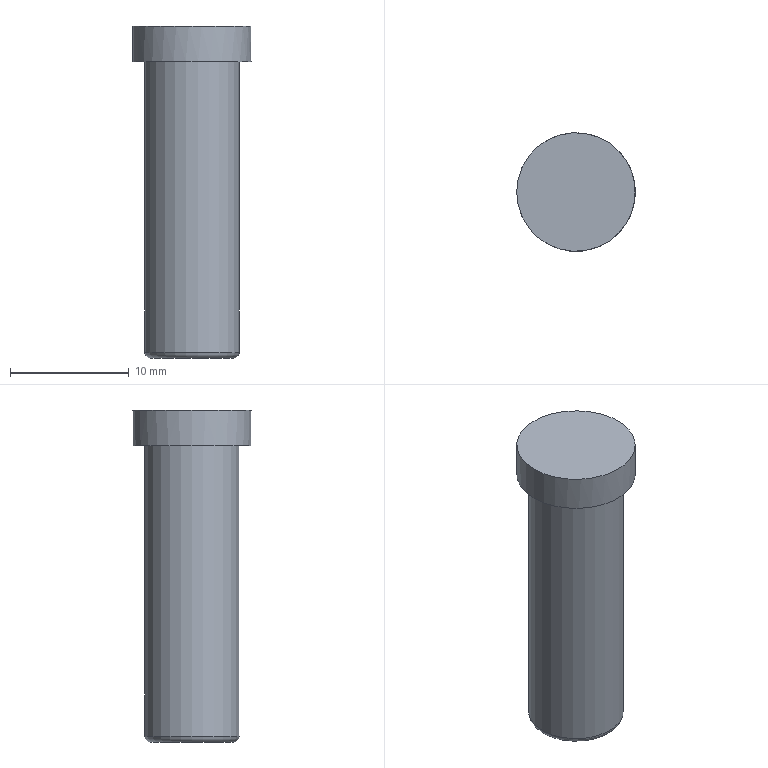Part | STEP file | lll_id2774_x_t | 1 solid | 6 faces | box 10 x 10 x 28 mm | volume 1491 mm3 | plane 3 | cylinder 2 | torus 1 | commonest cylinder face diameters 8 x1 10 x1
STEP:
#1=CARTESIAN_POINT('',(3587.5,0.,-2.5));
#2=VERTEX_POINT('',#1);
#3=CARTESIAN_POINT('',(3584.,0.,-2.5));
#4=DIRECTION('',(0.,0.,1.));
#5=DIRECTION('',(1.,0.,0.));
#6=AXIS2_PLACEMENT_3D('',#3,#4,#5);
#7=CIRCLE('',#6,3.5);
#8=EDGE_CURVE('',#2,#2,#7,.T.);
#9=ORIENTED_EDGE('',*,*,#8,.F.);
#10=EDGE_LOOP('',(#9));
#11=FACE_OUTER_BOUND('',#10,.T.);
#12=CARTESIAN_POINT('',(3584.,0.,-2.5));
#13=DIRECTION('',(0.,0.,-1.));
#14=DIRECTION('',(1.,0.,0.));
#15=AXIS2_PLACEMENT_3D('',#12,#13,#14);
#16=PLANE('',#15);
#17=ADVANCED_FACE('',(#11),#16,.T.);
#18=CARTESIAN_POINT('',(3588.,0.,22.5));
#19=VERTEX_POINT('',#18);
#20=CARTESIAN_POINT('',(3584.,0.,22.5));
#21=DIRECTION('',(0.,0.,-1.));
#22=DIRECTION('',(1.,0.,0.));
#23=AXIS2_PLACEMENT_3D('',#20,#21,#22);
#24=CIRCLE('',#23,4.);
#25=EDGE_CURVE('',#19,#19,#24,.T.);
#26=ORIENTED_EDGE('',*,*,#25,.T.);
#27=EDGE_LOOP('',(#26));
#28=FACE_BOUND('',#27,.T.);
#29=CARTESIAN_POINT('',(3588.,0.,-2.));
#30=VERTEX_POINT('',#29);
#31=CARTESIAN_POINT('',(3584.,0.,-2.));
#32=DIRECTION('',(0.,0.,-1.));
#33=DIRECTION('',(1.,0.,0.));
#34=AXIS2_PLACEMENT_3D('',#31,#32,#33);
#35=CIRCLE('',#34,4.);
#36=EDGE_CURVE('',#30,#30,#35,.T.);
#37=ORIENTED_EDGE('',*,*,#36,.F.);
#38=EDGE_LOOP('',(#37));
#39=FACE_BOUND('',#38,.T.);
#40=CARTESIAN_POINT('',(3584.,0.,30.5));
#41=DIRECTION('',(0.,0.,-1.));
#42=DIRECTION('',(-1.,0.,0.));
#43=AXIS2_PLACEMENT_3D('',#40,#41,#42);
#44=CYLINDRICAL_SURFACE('',#43,4.);
#45=ADVANCED_FACE('',(#28,#39),#44,.T.);
#46=ORIENTED_EDGE('',*,*,#8,.T.);
#47=EDGE_LOOP('',(#46));
#48=FACE_BOUND('',#47,.T.);
#49=ORIENTED_EDGE('',*,*,#36,.T.);
#50=EDGE_LOOP('',(#49));
#51=FACE_BOUND('',#50,.T.);
#52=CARTESIAN_POINT('',(3584.,0.,-2.));
#53=DIRECTION('',(0.,0.,-1.));
#54=DIRECTION('',(1.,0.,0.));
#55=AXIS2_PLACEMENT_3D('',#52,#53,#54);
#56=TOROIDAL_SURFACE('',#55,3.5,0.5);
#57=ADVANCED_FACE('',(#48,#51),#56,.T.);
#58=ORIENTED_EDGE('',*,*,#25,.F.);
#59=EDGE_LOOP('',(#58));
#60=FACE_BOUND('',#59,.T.);
#61=CARTESIAN_POINT('',(3589.,0.,22.5));
#62=VERTEX_POINT('',#61);
#63=CARTESIAN_POINT('',(3584.,0.,22.5));
#64=DIRECTION('',(0.,0.,-1.));
#65=DIRECTION('',(1.,0.,0.));
#66=AXIS2_PLACEMENT_3D('',#63,#64,#65);
#67=CIRCLE('',#66,5.);
#68=EDGE_CURVE('',#62,#62,#67,.T.);
#69=ORIENTED_EDGE('',*,*,#68,.T.);
#70=EDGE_LOOP('',(#69));
#71=FACE_BOUND('',#70,.T.);
#72=CARTESIAN_POINT('',(3584.,0.,22.5));
#73=DIRECTION('',(0.,0.,-1.));
#74=DIRECTION('',(1.,0.,0.));
#75=AXIS2_PLACEMENT_3D('',#72,#73,#74);
#76=PLANE('',#75);
#77=ADVANCED_FACE('',(#60,#71),#76,.T.);
#78=ORIENTED_EDGE('',*,*,#68,.F.);
#79=EDGE_LOOP('',(#78));
#80=FACE_BOUND('',#79,.T.);
#81=CARTESIAN_POINT('',(3579.,0.,25.5));
#82=VERTEX_POINT('',#81);
#83=CARTESIAN_POINT('',(3584.,0.,25.5));
#84=DIRECTION('',(0.,0.,1.));
#85=DIRECTION('',(-1.,0.,0.));
#86=AXIS2_PLACEMENT_3D('',#83,#84,#85);
#87=CIRCLE('',#86,5.);
#88=EDGE_CURVE('',#82,#82,#87,.T.);
#89=ORIENTED_EDGE('',*,*,#88,.F.);
#90=EDGE_LOOP('',(#89));
#91=FACE_BOUND('',#90,.T.);
#92=CARTESIAN_POINT('',(3584.,0.,25.5));
#93=DIRECTION('',(0.,0.,-1.));
#94=DIRECTION('',(-1.,0.,0.));
#95=AXIS2_PLACEMENT_3D('',#92,#93,#94);
#96=CYLINDRICAL_SURFACE('',#95,5.);
#97=ADVANCED_FACE('',(#80,#91),#96,.T.);
#98=ORIENTED_EDGE('',*,*,#88,.T.);
#99=EDGE_LOOP('',(#98));
#100=FACE_OUTER_BOUND('',#99,.T.);
#101=CARTESIAN_POINT('',(3584.,0.,25.5));
#102=DIRECTION('',(0.,0.,1.));
#103=DIRECTION('',(-1.,0.,0.));
#104=AXIS2_PLACEMENT_3D('',#101,#102,#103);
#105=PLANE('',#104);
#106=ADVANCED_FACE('',(#100),#105,.T.);
#107=CLOSED_SHELL('',(#17,#45,#57,#77,#97,#106));
#108=MANIFOLD_SOLID_BREP('',#107);
#109=(LENGTH_UNIT()NAMED_UNIT(*)SI_UNIT(.MILLI.,.METRE.));
#110=UNCERTAINTY_MEASURE_WITH_UNIT(LENGTH_MEASURE(0.00002),#109,'','');
#111=(NAMED_UNIT(*)PLANE_ANGLE_UNIT()SI_UNIT($,.RADIAN.));
#112=PLANE_ANGLE_MEASURE_WITH_UNIT(PLANE_ANGLE_MEASURE(0.01745),#111);
#113=DIMENSIONAL_EXPONENTS(0.,0.,0.,0.,0.,0.,0.);
#114=(CONVERSION_BASED_UNIT('DEGREE',#112)NAMED_UNIT(#113)PLANE_ANGLE_UNIT());
#115=(NAMED_UNIT(*)SI_UNIT($,.STERADIAN.)SOLID_ANGLE_UNIT());
#116=(GEOMETRIC_REPRESENTATION_CONTEXT(3)GLOBAL_UNCERTAINTY_ASSIGNED_CONTEXT((#110))GLOBAL_UNIT_ASSIGNED_CONTEXT((#109,#114,#115))REPRESENTATION_CONTEXT('',''));
#117=ADVANCED_BREP_SHAPE_REPRESENTATION('',(#108),#116);